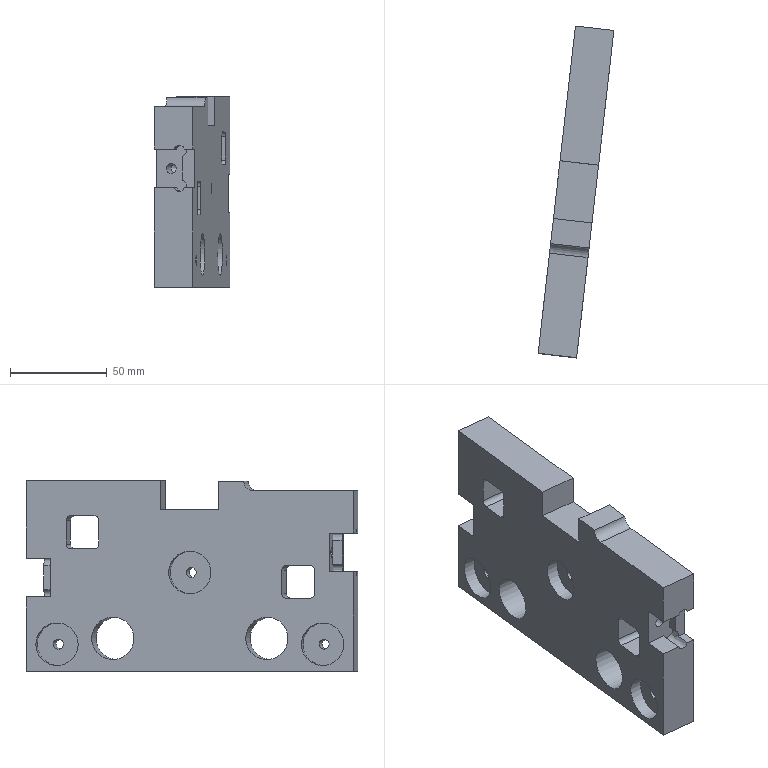Part | NX | features XQ 2 | 1 solid | 63 faces | box 39.116 x 171.171 x 98.374 mm | volume 274316 mm3 | plane 38 | cylinder 19 | spline 4 | cone 2 | commonest cylinder face diameters 5.08 x8 5.2 x5 22 x5 10 x1